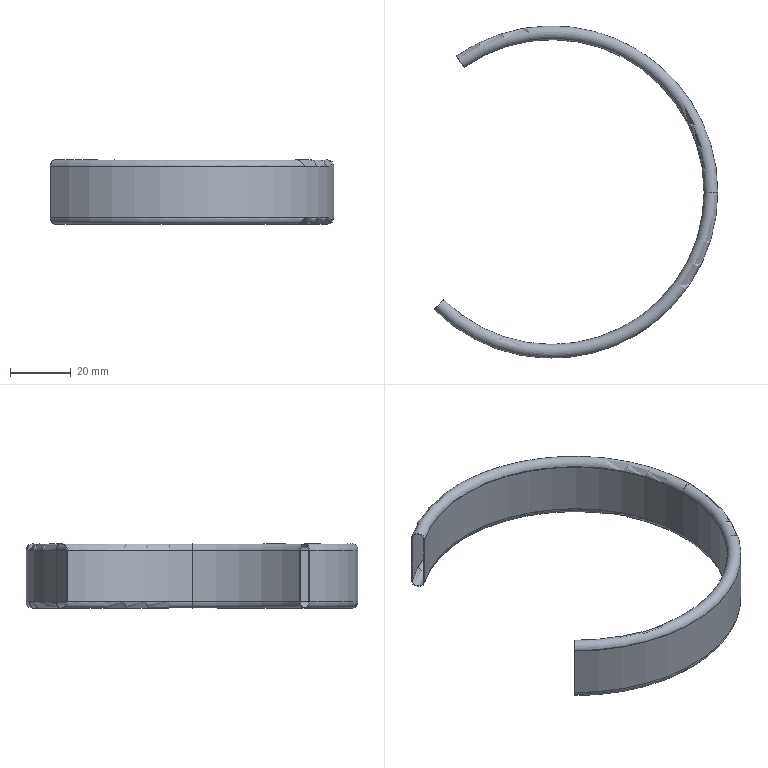Part | SolidWorks | features Sweep 1 | 1 solid | 18 faces | box 93.293 x 109.3 x 21.3 mm | volume 3338 mm3 | cylinder 8 | torus 8 | plane 2 | commonest cylinder face diameters 100.3 x2 100.9 x2 108.7 x2 109.3 x2
STEP:
#1=CARTESIAN_POINT('',(54.35,0.,-8.4));
#2=VERTEX_POINT('',#1);
#3=CARTESIAN_POINT('',(-31.174,44.521,-8.4));
#4=VERTEX_POINT('',#3);
#5=CARTESIAN_POINT('',(0.,0.,-8.4));
#6=DIRECTION('',(0.,0.,1.));
#7=DIRECTION('',(-0.7071,-0.7071,0.));
#8=AXIS2_PLACEMENT_3D('',#5,#6,#7);
#9=CIRCLE('',#8,54.35);
#10=EDGE_CURVE('',#2,#4,#9,.T.);
#11=ORIENTED_EDGE('',*,*,#10,.F.);
#12=CARTESIAN_POINT('',(54.35,0.,8.4));
#13=VERTEX_POINT('',#12);
#14=CARTESIAN_POINT('',(54.35,0.,0.));
#15=DIRECTION('',(0.,0.,1.));
#16=VECTOR('',#15,1000.);
#17=LINE('',#14,#16);
#18=EDGE_CURVE('',#2,#13,#17,.T.);
#19=ORIENTED_EDGE('',*,*,#18,.T.);
#20=CARTESIAN_POINT('',(-31.174,44.521,8.4));
#21=VERTEX_POINT('',#20);
#22=CARTESIAN_POINT('',(0.,0.,8.4));
#23=DIRECTION('',(0.,0.,1.));
#24=DIRECTION('',(-0.7071,-0.7071,0.));
#25=AXIS2_PLACEMENT_3D('',#22,#23,#24);
#26=CIRCLE('',#25,54.35);
#27=EDGE_CURVE('',#13,#21,#26,.T.);
#28=ORIENTED_EDGE('',*,*,#27,.T.);
#29=CARTESIAN_POINT('',(-31.174,44.521,-8.4));
#30=DIRECTION('',(0.,0.,-1.));
#31=VECTOR('',#30,1000.);
#32=LINE('',#29,#31);
#33=EDGE_CURVE('',#21,#4,#32,.T.);
#34=ORIENTED_EDGE('',*,*,#33,.T.);
#35=EDGE_LOOP('',(#11,#19,#28,#34));
#36=FACE_OUTER_BOUND('',#35,.T.);
#37=CARTESIAN_POINT('',(0.,0.,0.));
#38=DIRECTION('',(0.,0.,1.));
#39=DIRECTION('',(1.,0.,0.));
#40=AXIS2_PLACEMENT_3D('',#37,#38,#39);
#41=CYLINDRICAL_SURFACE('',#40,54.35);
#42=ADVANCED_FACE('',(#36),#41,.F.);
#43=ORIENTED_EDGE('',*,*,#27,.F.);
#44=CARTESIAN_POINT('',(50.45,0.,8.4));
#45=VERTEX_POINT('',#44);
#46=CARTESIAN_POINT('',(52.4,0.,8.4));
#47=DIRECTION('',(0.,-1.,0.));
#48=DIRECTION('',(0.,0.,-1.));
#49=AXIS2_PLACEMENT_3D('',#46,#47,#48);
#50=CIRCLE('',#49,1.95);
#51=EDGE_CURVE('',#13,#45,#50,.T.);
#52=ORIENTED_EDGE('',*,*,#51,.T.);
#53=CARTESIAN_POINT('',(-28.937,41.326,8.4));
#54=VERTEX_POINT('',#53);
#55=CARTESIAN_POINT('',(0.,0.,8.4));
#56=DIRECTION('',(0.,0.,1.));
#57=DIRECTION('',(-0.7071,-0.7071,0.));
#58=AXIS2_PLACEMENT_3D('',#55,#56,#57);
#59=CIRCLE('',#58,50.45);
#60=EDGE_CURVE('',#45,#54,#59,.T.);
#61=ORIENTED_EDGE('',*,*,#60,.T.);
#62=CARTESIAN_POINT('',(-30.055,42.924,8.4));
#63=DIRECTION('',(-0.8192,-0.5736,0.));
#64=DIRECTION('',(-0.5736,0.8192,0.));
#65=AXIS2_PLACEMENT_3D('',#62,#63,#64);
#66=CIRCLE('',#65,1.95);
#67=EDGE_CURVE('',#54,#21,#66,.T.);
#68=ORIENTED_EDGE('',*,*,#67,.T.);
#69=EDGE_LOOP('',(#43,#52,#61,#68));
#70=FACE_OUTER_BOUND('',#69,.T.);
#71=CARTESIAN_POINT('',(0.,0.,8.4));
#72=DIRECTION('',(0.,0.,1.));
#73=DIRECTION('',(1.,0.,0.));
#74=AXIS2_PLACEMENT_3D('',#71,#72,#73);
#75=TOROIDAL_SURFACE('',#74,52.4,1.95);
#76=ADVANCED_FACE('',(#70),#75,.F.);
#77=CARTESIAN_POINT('',(-35.674,-35.674,-8.4));
#78=VERTEX_POINT('',#77);
#79=CARTESIAN_POINT('',(50.45,0.,-8.4));
#80=VERTEX_POINT('',#79);
#81=CARTESIAN_POINT('',(0.,0.,-8.4));
#82=DIRECTION('',(0.,0.,1.));
#83=DIRECTION('',(-0.7071,-0.7071,0.));
#84=AXIS2_PLACEMENT_3D('',#81,#82,#83);
#85=CIRCLE('',#84,50.45);
#86=EDGE_CURVE('',#78,#80,#85,.T.);
#87=ORIENTED_EDGE('',*,*,#86,.T.);
#88=CARTESIAN_POINT('',(50.45,0.,0.));
#89=DIRECTION('',(0.,0.,1.));
#90=VECTOR('',#89,1000.);
#91=LINE('',#88,#90);
#92=EDGE_CURVE('',#80,#45,#91,.T.);
#93=ORIENTED_EDGE('',*,*,#92,.T.);
#94=CARTESIAN_POINT('',(-35.674,-35.674,8.4));
#95=VERTEX_POINT('',#94);
#96=CARTESIAN_POINT('',(0.,0.,8.4));
#97=DIRECTION('',(0.,0.,1.));
#98=DIRECTION('',(-0.7071,-0.7071,0.));
#99=AXIS2_PLACEMENT_3D('',#96,#97,#98);
#100=CIRCLE('',#99,50.45);
#101=EDGE_CURVE('',#95,#45,#100,.T.);
#102=ORIENTED_EDGE('',*,*,#101,.F.);
#103=CARTESIAN_POINT('',(-35.674,-35.674,-8.4));
#104=DIRECTION('',(0.,0.,1.));
#105=VECTOR('',#104,1000.);
#106=LINE('',#103,#105);
#107=EDGE_CURVE('',#78,#95,#106,.T.);
#108=ORIENTED_EDGE('',*,*,#107,.F.);
#109=EDGE_LOOP('',(#87,#93,#102,#108));
#110=FACE_OUTER_BOUND('',#109,.T.);
#111=CARTESIAN_POINT('',(0.,0.,0.));
#112=DIRECTION('',(0.,0.,1.));
#113=DIRECTION('',(1.,0.,0.));
#114=AXIS2_PLACEMENT_3D('',#111,#112,#113);
#115=CYLINDRICAL_SURFACE('',#114,50.45);
#116=ADVANCED_FACE('',(#110),#115,.T.);
#117=CARTESIAN_POINT('',(-28.937,41.326,-8.4));
#118=VERTEX_POINT('',#117);
#119=CARTESIAN_POINT('',(0.,0.,-8.4));
#120=DIRECTION('',(0.,0.,1.));
#121=DIRECTION('',(-0.7071,-0.7071,0.));
#122=AXIS2_PLACEMENT_3D('',#119,#120,#121);
#123=CIRCLE('',#122,50.45);
#124=EDGE_CURVE('',#80,#118,#123,.T.);
#125=ORIENTED_EDGE('',*,*,#124,.F.);
#126=CARTESIAN_POINT('',(52.4,0.,-8.4));
#127=DIRECTION('',(0.,-1.,0.));
#128=DIRECTION('',(0.,0.,-1.));
#129=AXIS2_PLACEMENT_3D('',#126,#127,#128);
#130=CIRCLE('',#129,1.95);
#131=EDGE_CURVE('',#80,#2,#130,.T.);
#132=ORIENTED_EDGE('',*,*,#131,.T.);
#133=ORIENTED_EDGE('',*,*,#10,.T.);
#134=CARTESIAN_POINT('',(-30.055,42.924,-8.4));
#135=DIRECTION('',(-0.8192,-0.5736,0.));
#136=DIRECTION('',(-0.5736,0.8192,0.));
#137=AXIS2_PLACEMENT_3D('',#134,#135,#136);
#138=CIRCLE('',#137,1.95);
#139=EDGE_CURVE('',#4,#118,#138,.T.);
#140=ORIENTED_EDGE('',*,*,#139,.T.);
#141=EDGE_LOOP('',(#125,#132,#133,#140));
#142=FACE_OUTER_BOUND('',#141,.T.);
#143=CARTESIAN_POINT('',(0.,0.,-8.4));
#144=DIRECTION('',(0.,0.,1.));
#145=DIRECTION('',(1.,0.,0.));
#146=AXIS2_PLACEMENT_3D('',#143,#144,#145);
#147=TOROIDAL_SURFACE('',#146,52.4,1.95);
#148=ADVANCED_FACE('',(#142),#147,.F.);
#149=CARTESIAN_POINT('',(-38.643,-38.643,8.4));
#150=VERTEX_POINT('',#149);
#151=CARTESIAN_POINT('',(54.65,0.,8.4));
#152=VERTEX_POINT('',#151);
#153=CARTESIAN_POINT('',(0.,0.,8.4));
#154=DIRECTION('',(0.,0.,1.));
#155=DIRECTION('',(-0.7071,-0.7071,0.));
#156=AXIS2_PLACEMENT_3D('',#153,#154,#155);
#157=CIRCLE('',#156,54.65);
#158=EDGE_CURVE('',#150,#152,#157,.T.);
#159=ORIENTED_EDGE('',*,*,#158,.T.);
#160=CARTESIAN_POINT('',(50.15,0.,8.4));
#161=VERTEX_POINT('',#160);
#162=CARTESIAN_POINT('',(52.4,0.,8.4));
#163=DIRECTION('',(0.,-1.,0.));
#164=DIRECTION('',(0.,0.,-1.));
#165=AXIS2_PLACEMENT_3D('',#162,#163,#164);
#166=CIRCLE('',#165,2.25);
#167=EDGE_CURVE('',#152,#161,#166,.T.);
#168=ORIENTED_EDGE('',*,*,#167,.T.);
#169=CARTESIAN_POINT('',(-35.461,-35.461,8.4));
#170=VERTEX_POINT('',#169);
#171=CARTESIAN_POINT('',(0.,0.,8.4));
#172=DIRECTION('',(0.,0.,1.));
#173=DIRECTION('',(-0.7071,-0.7071,0.));
#174=AXIS2_PLACEMENT_3D('',#171,#172,#173);
#175=CIRCLE('',#174,50.15);
#176=EDGE_CURVE('',#170,#161,#175,.T.);
#177=ORIENTED_EDGE('',*,*,#176,.F.);
#178=CARTESIAN_POINT('',(-37.052,-37.052,8.4));
#179=DIRECTION('',(-0.7071,0.7071,0.));
#180=DIRECTION('',(-0.7071,-0.7071,0.));
#181=AXIS2_PLACEMENT_3D('',#178,#179,#180);
#182=CIRCLE('',#181,2.25);
#183=EDGE_CURVE('',#150,#170,#182,.T.);
#184=ORIENTED_EDGE('',*,*,#183,.F.);
#185=EDGE_LOOP('',(#159,#168,#177,#184));
#186=FACE_OUTER_BOUND('',#185,.T.);
#187=CARTESIAN_POINT('',(0.,0.,8.4));
#188=DIRECTION('',(0.,0.,1.));
#189=DIRECTION('',(1.,0.,0.));
#190=AXIS2_PLACEMENT_3D('',#187,#188,#189);
#191=TOROIDAL_SURFACE('',#190,52.4,2.25);
#192=ADVANCED_FACE('',(#186),#191,.T.);
#193=CARTESIAN_POINT('',(-38.643,-38.643,-8.4));
#194=VERTEX_POINT('',#193);
#195=CARTESIAN_POINT('',(54.65,0.,-8.4));
#196=VERTEX_POINT('',#195);
#197=CARTESIAN_POINT('',(0.,0.,-8.4));
#198=DIRECTION('',(0.,0.,1.));
#199=DIRECTION('',(-0.7071,-0.7071,0.));
#200=AXIS2_PLACEMENT_3D('',#197,#198,#199);
#201=CIRCLE('',#200,54.65);
#202=EDGE_CURVE('',#194,#196,#201,.T.);
#203=ORIENTED_EDGE('',*,*,#202,.T.);
#204=CARTESIAN_POINT('',(54.65,0.,0.));
#205=DIRECTION('',(0.,0.,1.));
#206=VECTOR('',#205,1000.);
#207=LINE('',#204,#206);
#208=EDGE_CURVE('',#196,#152,#207,.T.);
#209=ORIENTED_EDGE('',*,*,#208,.T.);
#210=ORIENTED_EDGE('',*,*,#158,.F.);
#211=CARTESIAN_POINT('',(-38.643,-38.643,-8.4));
#212=DIRECTION('',(0.,0.,1.));
#213=VECTOR('',#212,1000.);
#214=LINE('',#211,#213);
#215=EDGE_CURVE('',#194,#150,#214,.T.);
#216=ORIENTED_EDGE('',*,*,#215,.F.);
#217=EDGE_LOOP('',(#203,#209,#210,#216));
#218=FACE_OUTER_BOUND('',#217,.T.);
#219=CARTESIAN_POINT('',(0.,0.,0.));
#220=DIRECTION('',(0.,0.,1.));
#221=DIRECTION('',(1.,0.,0.));
#222=AXIS2_PLACEMENT_3D('',#219,#220,#221);
#223=CYLINDRICAL_SURFACE('',#222,54.65);
#224=ADVANCED_FACE('',(#218),#223,.T.);
#225=CARTESIAN_POINT('',(-35.461,-35.461,-8.4));
#226=VERTEX_POINT('',#225);
#227=CARTESIAN_POINT('',(50.15,0.,-8.4));
#228=VERTEX_POINT('',#227);
#229=CARTESIAN_POINT('',(0.,0.,-8.4));
#230=DIRECTION('',(0.,0.,1.));
#231=DIRECTION('',(-0.7071,-0.7071,0.));
#232=AXIS2_PLACEMENT_3D('',#229,#230,#231);
#233=CIRCLE('',#232,50.15);
#234=EDGE_CURVE('',#226,#228,#233,.T.);
#235=ORIENTED_EDGE('',*,*,#234,.T.);
#236=CARTESIAN_POINT('',(52.4,0.,-8.4));
#237=DIRECTION('',(0.,-1.,0.));
#238=DIRECTION('',(0.,0.,-1.));
#239=AXIS2_PLACEMENT_3D('',#236,#237,#238);
#240=CIRCLE('',#239,2.25);
#241=EDGE_CURVE('',#228,#196,#240,.T.);
#242=ORIENTED_EDGE('',*,*,#241,.T.);
#243=ORIENTED_EDGE('',*,*,#202,.F.);
#244=CARTESIAN_POINT('',(-37.052,-37.052,-8.4));
#245=DIRECTION('',(-0.7071,0.7071,0.));
#246=DIRECTION('',(-0.7071,-0.7071,0.));
#247=AXIS2_PLACEMENT_3D('',#244,#245,#246);
#248=CIRCLE('',#247,2.25);
#249=EDGE_CURVE('',#226,#194,#248,.T.);
#250=ORIENTED_EDGE('',*,*,#249,.F.);
#251=EDGE_LOOP('',(#235,#242,#243,#250));
#252=FACE_OUTER_BOUND('',#251,.T.);
#253=CARTESIAN_POINT('',(0.,0.,-8.4));
#254=DIRECTION('',(0.,0.,1.));
#255=DIRECTION('',(1.,0.,0.));
#256=AXIS2_PLACEMENT_3D('',#253,#254,#255);
#257=TOROIDAL_SURFACE('',#256,52.4,2.25);
#258=ADVANCED_FACE('',(#252),#257,.T.);
#259=CARTESIAN_POINT('',(-28.765,41.08,-8.4));
#260=VERTEX_POINT('',#259);
#261=CARTESIAN_POINT('',(0.,0.,-8.4));
#262=DIRECTION('',(0.,0.,1.));
#263=DIRECTION('',(-0.7071,-0.7071,0.));
#264=AXIS2_PLACEMENT_3D('',#261,#262,#263);
#265=CIRCLE('',#264,50.15);
#266=EDGE_CURVE('',#228,#260,#265,.T.);
#267=ORIENTED_EDGE('',*,*,#266,.F.);
#268=CARTESIAN_POINT('',(50.15,0.,0.));
#269=DIRECTION('',(0.,0.,1.));
#270=VECTOR('',#269,1000.);
#271=LINE('',#268,#270);
#272=EDGE_CURVE('',#228,#161,#271,.T.);
#273=ORIENTED_EDGE('',*,*,#272,.T.);
#274=CARTESIAN_POINT('',(-28.765,41.08,8.4));
#275=VERTEX_POINT('',#274);
#276=CARTESIAN_POINT('',(0.,0.,8.4));
#277=DIRECTION('',(0.,0.,1.));
#278=DIRECTION('',(-0.7071,-0.7071,0.));
#279=AXIS2_PLACEMENT_3D('',#276,#277,#278);
#280=CIRCLE('',#279,50.15);
#281=EDGE_CURVE('',#161,#275,#280,.T.);
#282=ORIENTED_EDGE('',*,*,#281,.T.);
#283=CARTESIAN_POINT('',(-28.765,41.08,-8.4));
#284=DIRECTION('',(0.,0.,-1.));
#285=VECTOR('',#284,1000.);
#286=LINE('',#283,#285);
#287=EDGE_CURVE('',#275,#260,#286,.T.);
#288=ORIENTED_EDGE('',*,*,#287,.T.);
#289=EDGE_LOOP('',(#267,#273,#282,#288));
#290=FACE_OUTER_BOUND('',#289,.T.);
#291=CARTESIAN_POINT('',(0.,0.,0.));
#292=DIRECTION('',(0.,0.,1.));
#293=DIRECTION('',(1.,0.,0.));
#294=AXIS2_PLACEMENT_3D('',#291,#292,#293);
#295=CYLINDRICAL_SURFACE('',#294,50.15);
#296=ADVANCED_FACE('',(#290),#295,.F.);
#297=ORIENTED_EDGE('',*,*,#18,.F.);
#298=CARTESIAN_POINT('',(-38.431,-38.431,-8.4));
#299=VERTEX_POINT('',#298);
#300=CARTESIAN_POINT('',(0.,0.,-8.4));
#301=DIRECTION('',(0.,0.,1.));
#302=DIRECTION('',(-0.7071,-0.7071,0.));
#303=AXIS2_PLACEMENT_3D('',#300,#301,#302);
#304=CIRCLE('',#303,54.35);
#305=EDGE_CURVE('',#299,#2,#304,.T.);
#306=ORIENTED_EDGE('',*,*,#305,.F.);
#307=CARTESIAN_POINT('',(-38.431,-38.431,8.4));
#308=VERTEX_POINT('',#307);
#309=CARTESIAN_POINT('',(-38.431,-38.431,-8.4));
#310=DIRECTION('',(0.,0.,-1.));
#311=VECTOR('',#310,1000.);
#312=LINE('',#309,#311);
#313=EDGE_CURVE('',#308,#299,#312,.T.);
#314=ORIENTED_EDGE('',*,*,#313,.F.);
#315=CARTESIAN_POINT('',(0.,0.,8.4));
#316=DIRECTION('',(0.,0.,1.));
#317=DIRECTION('',(-0.7071,-0.7071,0.));
#318=AXIS2_PLACEMENT_3D('',#315,#316,#317);
#319=CIRCLE('',#318,54.35);
#320=EDGE_CURVE('',#308,#13,#319,.T.);
#321=ORIENTED_EDGE('',*,*,#320,.T.);
#322=EDGE_LOOP('',(#297,#306,#314,#321));
#323=FACE_OUTER_BOUND('',#322,.T.);
#324=CARTESIAN_POINT('',(0.,0.,0.));
#325=DIRECTION('',(0.,0.,1.));
#326=DIRECTION('',(1.,0.,0.));
#327=AXIS2_PLACEMENT_3D('',#324,#325,#326);
#328=CYLINDRICAL_SURFACE('',#327,54.35);
#329=ADVANCED_FACE('',(#323),#328,.F.);
#330=ORIENTED_EDGE('',*,*,#51,.F.);
#331=ORIENTED_EDGE('',*,*,#320,.F.);
#332=CARTESIAN_POINT('',(-37.052,-37.052,8.4));
#333=DIRECTION('',(0.7071,-0.7071,0.));
#334=DIRECTION('',(-0.7071,-0.7071,0.));
#335=AXIS2_PLACEMENT_3D('',#332,#333,#334);
#336=CIRCLE('',#335,1.95);
#337=EDGE_CURVE('',#95,#308,#336,.T.);
#338=ORIENTED_EDGE('',*,*,#337,.F.);
#339=ORIENTED_EDGE('',*,*,#101,.T.);
#340=EDGE_LOOP('',(#330,#331,#338,#339));
#341=FACE_OUTER_BOUND('',#340,.T.);
#342=CARTESIAN_POINT('',(0.,0.,8.4));
#343=DIRECTION('',(0.,0.,1.));
#344=DIRECTION('',(1.,0.,0.));
#345=AXIS2_PLACEMENT_3D('',#342,#343,#344);
#346=TOROIDAL_SURFACE('',#345,52.4,1.95);
#347=ADVANCED_FACE('',(#341),#346,.F.);
#348=ORIENTED_EDGE('',*,*,#92,.F.);
#349=ORIENTED_EDGE('',*,*,#124,.T.);
#350=CARTESIAN_POINT('',(-28.937,41.326,-8.4));
#351=DIRECTION('',(0.,0.,1.));
#352=VECTOR('',#351,1000.);
#353=LINE('',#350,#352);
#354=EDGE_CURVE('',#118,#54,#353,.T.);
#355=ORIENTED_EDGE('',*,*,#354,.T.);
#356=ORIENTED_EDGE('',*,*,#60,.F.);
#357=EDGE_LOOP('',(#348,#349,#355,#356));
#358=FACE_OUTER_BOUND('',#357,.T.);
#359=CARTESIAN_POINT('',(0.,0.,0.));
#360=DIRECTION('',(0.,0.,1.));
#361=DIRECTION('',(1.,0.,0.));
#362=AXIS2_PLACEMENT_3D('',#359,#360,#361);
#363=CYLINDRICAL_SURFACE('',#362,50.45);
#364=ADVANCED_FACE('',(#358),#363,.T.);
#365=ORIENTED_EDGE('',*,*,#131,.F.);
#366=ORIENTED_EDGE('',*,*,#86,.F.);
#367=CARTESIAN_POINT('',(-37.052,-37.052,-8.4));
#368=DIRECTION('',(0.7071,-0.7071,0.));
#369=DIRECTION('',(-0.7071,-0.7071,0.));
#370=AXIS2_PLACEMENT_3D('',#367,#368,#369);
#371=CIRCLE('',#370,1.95);
#372=EDGE_CURVE('',#299,#78,#371,.T.);
#373=ORIENTED_EDGE('',*,*,#372,.F.);
#374=ORIENTED_EDGE('',*,*,#305,.T.);
#375=EDGE_LOOP('',(#365,#366,#373,#374));
#376=FACE_OUTER_BOUND('',#375,.T.);
#377=CARTESIAN_POINT('',(0.,0.,-8.4));
#378=DIRECTION('',(0.,0.,1.));
#379=DIRECTION('',(1.,0.,0.));
#380=AXIS2_PLACEMENT_3D('',#377,#378,#379);
#381=TOROIDAL_SURFACE('',#380,52.4,1.95);
#382=ADVANCED_FACE('',(#376),#381,.F.);
#383=ORIENTED_EDGE('',*,*,#139,.F.);
#384=ORIENTED_EDGE('',*,*,#33,.F.);
#385=ORIENTED_EDGE('',*,*,#67,.F.);
#386=ORIENTED_EDGE('',*,*,#354,.F.);
#387=EDGE_LOOP('',(#383,#384,#385,#386));
#388=FACE_BOUND('',#387,.T.);
#389=CARTESIAN_POINT('',(-31.346,44.767,-8.4));
#390=VERTEX_POINT('',#389);
#391=CARTESIAN_POINT('',(-30.055,42.924,-8.4));
#392=DIRECTION('',(0.8192,0.5736,0.));
#393=DIRECTION('',(-0.5736,0.8192,0.));
#394=AXIS2_PLACEMENT_3D('',#391,#392,#393);
#395=CIRCLE('',#394,2.25);
#396=EDGE_CURVE('',#260,#390,#395,.T.);
#397=ORIENTED_EDGE('',*,*,#396,.F.);
#398=ORIENTED_EDGE('',*,*,#287,.F.);
#399=CARTESIAN_POINT('',(-31.346,44.767,8.4));
#400=VERTEX_POINT('',#399);
#401=CARTESIAN_POINT('',(-30.055,42.924,8.4));
#402=DIRECTION('',(0.8192,0.5736,0.));
#403=DIRECTION('',(-0.5736,0.8192,0.));
#404=AXIS2_PLACEMENT_3D('',#401,#402,#403);
#405=CIRCLE('',#404,2.25);
#406=EDGE_CURVE('',#400,#275,#405,.T.);
#407=ORIENTED_EDGE('',*,*,#406,.F.);
#408=CARTESIAN_POINT('',(-31.346,44.767,-8.4));
#409=DIRECTION('',(0.,0.,1.));
#410=VECTOR('',#409,1000.);
#411=LINE('',#408,#410);
#412=EDGE_CURVE('',#390,#400,#411,.T.);
#413=ORIENTED_EDGE('',*,*,#412,.F.);
#414=EDGE_LOOP('',(#397,#398,#407,#413));
#415=FACE_OUTER_BOUND('',#414,.T.);
#416=CARTESIAN_POINT('',(-30.055,42.924,-8.4));
#417=DIRECTION('',(0.8192,0.5736,0.));
#418=DIRECTION('',(-0.5736,0.8192,0.));
#419=AXIS2_PLACEMENT_3D('',#416,#417,#418);
#420=PLANE('',#419);
#421=ADVANCED_FACE('',(#388,#415),#420,.F.);
#422=ORIENTED_EDGE('',*,*,#372,.T.);
#423=ORIENTED_EDGE('',*,*,#107,.T.);
#424=ORIENTED_EDGE('',*,*,#337,.T.);
#425=ORIENTED_EDGE('',*,*,#313,.T.);
#426=EDGE_LOOP('',(#422,#423,#424,#425));
#427=FACE_BOUND('',#426,.T.);
#428=ORIENTED_EDGE('',*,*,#249,.T.);
#429=ORIENTED_EDGE('',*,*,#215,.T.);
#430=ORIENTED_EDGE('',*,*,#183,.T.);
#431=CARTESIAN_POINT('',(-35.461,-35.461,-8.4));
#432=DIRECTION('',(0.,0.,-1.));
#433=VECTOR('',#432,1000.);
#434=LINE('',#431,#433);
#435=EDGE_CURVE('',#170,#226,#434,.T.);
#436=ORIENTED_EDGE('',*,*,#435,.T.);
#437=EDGE_LOOP('',(#428,#429,#430,#436));
#438=FACE_OUTER_BOUND('',#437,.T.);
#439=CARTESIAN_POINT('',(-37.052,-37.052,-8.4));
#440=DIRECTION('',(-0.7071,0.7071,0.));
#441=DIRECTION('',(-0.7071,-0.7071,0.));
#442=AXIS2_PLACEMENT_3D('',#439,#440,#441);
#443=PLANE('',#442);
#444=ADVANCED_FACE('',(#427,#438),#443,.T.);
#445=ORIENTED_EDGE('',*,*,#167,.F.);
#446=CARTESIAN_POINT('',(0.,0.,8.4));
#447=DIRECTION('',(0.,0.,1.));
#448=DIRECTION('',(-0.7071,-0.7071,0.));
#449=AXIS2_PLACEMENT_3D('',#446,#447,#448);
#450=CIRCLE('',#449,54.65);
#451=EDGE_CURVE('',#152,#400,#450,.T.);
#452=ORIENTED_EDGE('',*,*,#451,.T.);
#453=ORIENTED_EDGE('',*,*,#406,.T.);
#454=ORIENTED_EDGE('',*,*,#281,.F.);
#455=EDGE_LOOP('',(#445,#452,#453,#454));
#456=FACE_OUTER_BOUND('',#455,.T.);
#457=CARTESIAN_POINT('',(0.,0.,8.4));
#458=DIRECTION('',(0.,0.,1.));
#459=DIRECTION('',(1.,0.,0.));
#460=AXIS2_PLACEMENT_3D('',#457,#458,#459);
#461=TOROIDAL_SURFACE('',#460,52.4,2.25);
#462=ADVANCED_FACE('',(#456),#461,.T.);
#463=ORIENTED_EDGE('',*,*,#208,.F.);
#464=CARTESIAN_POINT('',(0.,0.,-8.4));
#465=DIRECTION('',(0.,0.,1.));
#466=DIRECTION('',(-0.7071,-0.7071,0.));
#467=AXIS2_PLACEMENT_3D('',#464,#465,#466);
#468=CIRCLE('',#467,54.65);
#469=EDGE_CURVE('',#196,#390,#468,.T.);
#470=ORIENTED_EDGE('',*,*,#469,.T.);
#471=ORIENTED_EDGE('',*,*,#412,.T.);
#472=ORIENTED_EDGE('',*,*,#451,.F.);
#473=EDGE_LOOP('',(#463,#470,#471,#472));
#474=FACE_OUTER_BOUND('',#473,.T.);
#475=CARTESIAN_POINT('',(0.,0.,0.));
#476=DIRECTION('',(0.,0.,1.));
#477=DIRECTION('',(1.,0.,0.));
#478=AXIS2_PLACEMENT_3D('',#475,#476,#477);
#479=CYLINDRICAL_SURFACE('',#478,54.65);
#480=ADVANCED_FACE('',(#474),#479,.T.);
#481=ORIENTED_EDGE('',*,*,#241,.F.);
#482=ORIENTED_EDGE('',*,*,#266,.T.);
#483=ORIENTED_EDGE('',*,*,#396,.T.);
#484=ORIENTED_EDGE('',*,*,#469,.F.);
#485=EDGE_LOOP('',(#481,#482,#483,#484));
#486=FACE_OUTER_BOUND('',#485,.T.);
#487=CARTESIAN_POINT('',(0.,0.,-8.4));
#488=DIRECTION('',(0.,0.,1.));
#489=DIRECTION('',(1.,0.,0.));
#490=AXIS2_PLACEMENT_3D('',#487,#488,#489);
#491=TOROIDAL_SURFACE('',#490,52.4,2.25);
#492=ADVANCED_FACE('',(#486),#491,.T.);
#493=ORIENTED_EDGE('',*,*,#272,.F.);
#494=ORIENTED_EDGE('',*,*,#234,.F.);
#495=ORIENTED_EDGE('',*,*,#435,.F.);
#496=ORIENTED_EDGE('',*,*,#176,.T.);
#497=EDGE_LOOP('',(#493,#494,#495,#496));
#498=FACE_OUTER_BOUND('',#497,.T.);
#499=CARTESIAN_POINT('',(0.,0.,0.));
#500=DIRECTION('',(0.,0.,1.));
#501=DIRECTION('',(1.,0.,0.));
#502=AXIS2_PLACEMENT_3D('',#499,#500,#501);
#503=CYLINDRICAL_SURFACE('',#502,50.15);
#504=ADVANCED_FACE('',(#498),#503,.F.);
#505=CLOSED_SHELL('',(#42,#76,#116,#148,#192,#224,#258,#296,#329,#347,#364,#382,#421,#444,#462,#480,#492,#504));
#506=MANIFOLD_SOLID_BREP('',#505);
#507=CARTESIAN_POINT('',(0.,0.,0.));
#508=DIRECTION('',(0.,0.,1.));
#509=DIRECTION('',(1.,0.,0.));
#510=AXIS2_PLACEMENT_3D('',#507,#508,#509);
#511=(LENGTH_UNIT()NAMED_UNIT(*)SI_UNIT(.MILLI.,.METRE.));
#512=UNCERTAINTY_MEASURE_WITH_UNIT(LENGTH_MEASURE(0.00001),#511,'','');
#513=(NAMED_UNIT(*)PLANE_ANGLE_UNIT()SI_UNIT($,.RADIAN.));
#514=(NAMED_UNIT(*)SI_UNIT($,.STERADIAN.)SOLID_ANGLE_UNIT());
#515=(GEOMETRIC_REPRESENTATION_CONTEXT(3)GLOBAL_UNCERTAINTY_ASSIGNED_CONTEXT((#512))GLOBAL_UNIT_ASSIGNED_CONTEXT((#511,#513,#514))REPRESENTATION_CONTEXT('',''));
#516=ADVANCED_BREP_SHAPE_REPRESENTATION('',(#506,#510),#515);